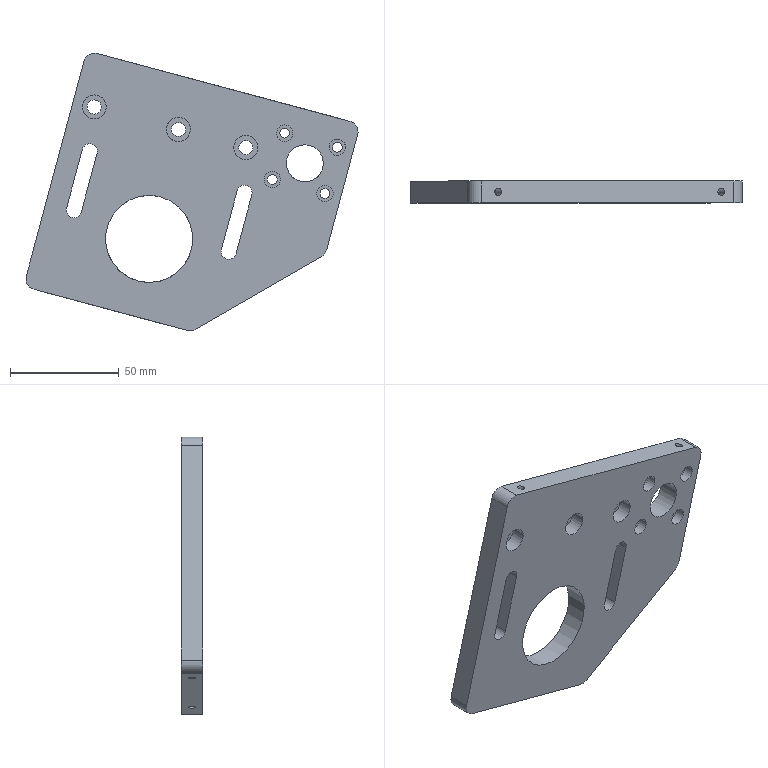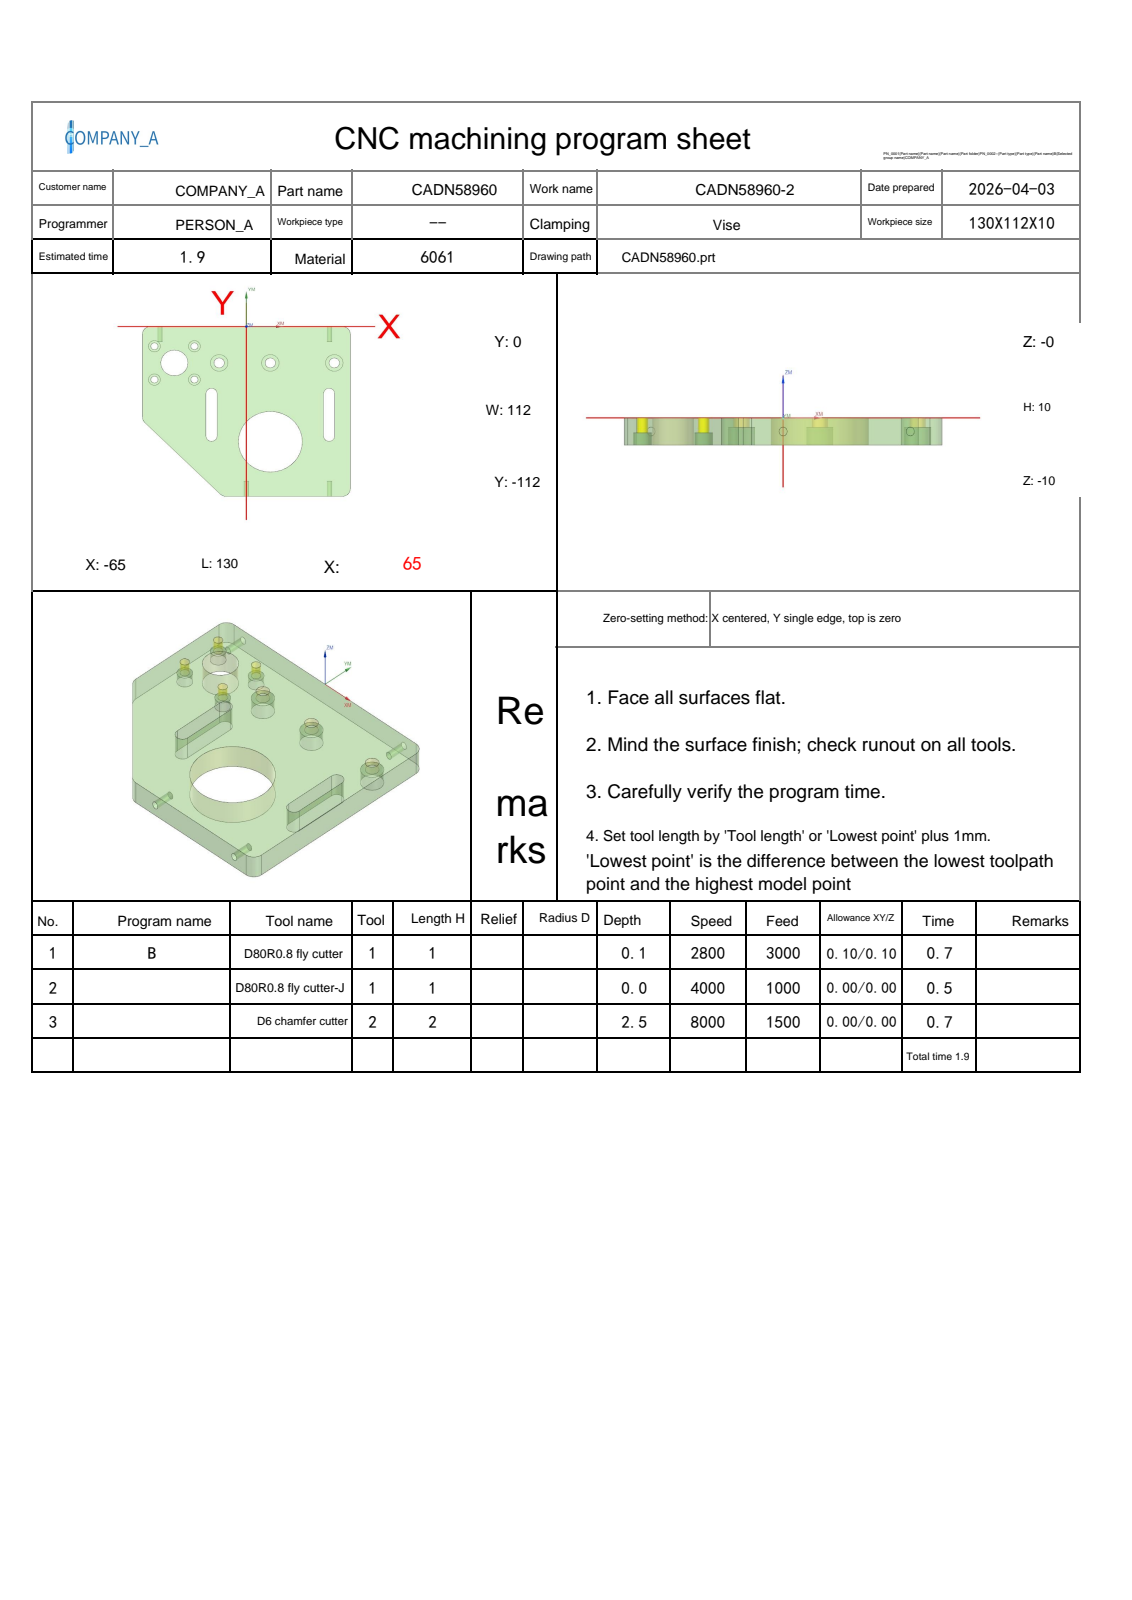NC program | NX | posted by the shop | part box 152.311 x 10 x 127.359 mm
Whole program:
%
O0001
(Machine time: 2.46 MIN)
(===Total Tool:2===)
(T1=D80R0.8 fly cutter D=80.  R=0.8  D-  H01 Z=-0.   )
(T2=D6 chamfer cutter   D=6.   R=0.   D-  H02 Z=-2.55 )
G80 G90 G17 G49 G40
G91 G28 Z0
M01
N1 T01 M06
(D80R0.8 fly cutter  D=80. R=0.8 H=01 ce=0.10 di=0.10)
G00 G90 G54 X117.097 Y-86.978 M03 S2800
G43 H01 Z20.
M08
Z3.525
G01 Z1.525 F3000.
X105.097 Y-87.213
X-88.772 Y-90.998
X-88.926 Y-90.999
G02 X-95.161 Y-88.011 I0.0 J8.
X-105.097 Y-59.772 I35.161 J28.239
G01 Y-39.991
G02 X-97.256 Y-31.996 I8. J-.003
G01 X105.097 Y-28.045
X117.097 Y-27.811
Z3.525
G00 Y-86.978
Z3.05
G01 Z1.05
X105.097 Y-87.213
X-88.772 Y-90.998
X-88.926 Y-90.999
G02 X-95.161 Y-88.011 I0.0 J8.
X-105.097 Y-59.772 I35.161 J28.239
G01 Y-39.991
G02 X-97.256 Y-31.996 I8. J-.003
G01 X105.097 Y-28.045
X117.097 Y-27.811
Z3.05
G00 Y-86.978
Z2.575
G01 Z.575
X105.097 Y-87.213
X-88.772 Y-90.998
X-88.926 Y-90.999
G02 X-95.161 Y-88.011 I0.0 J8.
X-105.097 Y-59.772 I35.161 J28.239
G01 Y-39.991
G02 X-97.256 Y-31.996 I8. J-.003
G01 X105.097 Y-28.045
X117.097 Y-27.811
Z2.575
G00 Y-86.978
Z2.1
G01 Z.1
X105.097 Y-87.213
X-88.772 Y-90.998
X-88.926 Y-90.999
G02 X-95.161 Y-88.011 I0.0 J8.
X-105.097 Y-59.772 I35.161 J28.239
G01 Y-39.991
G02 X-97.256 Y-31.996 I8. J-.003
G01 X105.097 Y-28.045
X117.097 Y-27.811
Z2.1
G00 Z20.
G91 G28 Z0.0
M05
M09
G91 G28 Z0.0
M01
N2 T01 M06
(D80R0.8 fly cutter-J  D=80. R=0.8 H=01 ce=0.00 di=0.00)
G00 G90 G54 X116.999 Y-86.884 M03 S4000
G43 H01 Z20.
M08
Z2.
G01 Z0.0 F1000.
X104.999 Y-87.118
X-88.729 Y-90.896
X-88.882 Y-90.897
G02 X-95.124 Y-87.9 I0.0 J8.
X-104.999 Y-59.772 I35.124 J28.128
G01 Y-40.087
G02 X-97.158 Y-32.091 I8. J-.003
G01 X104.999 Y-28.148
X116.999 Y-27.914
Z2.
G00 Z20.
G91 G28 Z0.0
M05
M09
G91 G28 Z0.0
M01
N3 T02 M06
(D6 chamfer cutter  D=6. R=0. H=02 ce=0.00 di=0.00)
G00 G90 G54 X-32.5 Y-35. M03 S8000
G43 H02 Z20.
M08
G98 G81 X-32.5 Y-35. Z-2.55 R3. F1000.
Y-13.
X-57.5
Y-35.
G80
G00 Z20.
G00 G90 X-.386 Y1.227 M03 S6500
Z20.
Z.172
G01 Z-1.499 F1500.
G03 X-.1 Y1.027 I1.286 J1.532
G01 X-.054 Y.997
X0.0 Y1.
X60.
G02 X66. Y-5. I0.0 J-6.
G01 Y-107.
G02 X60. Y-113. I-6. J0.0
G01 X-12.772
G02 X-17.015 Y-111.243 I0.0 J6.
G01 X-64.242 Y-64.015
G02 X-66. Y-59.772 I4.242 J4.243
G01 Y-5.
G02 X-60. Y1. I6. J0.0
G01 X0.0
X.054 Y.997
X.1 Y1.027
G03 X.386 Y1.227 I-1. J1.732
G01 Z.172
G00 Z10.
X9.759 Y-94.032
Z.198
G01 Z-1.499
G03 X9.991 Y-94.292 I1.602 J1.197
G01 X10.029 Y-94.332
X10.082 Y-94.341
G03 X15. Y-94.989 I4.918 J18.353
X34. Y-75.989 I0.0 J19.
X15. Y-56.989 I-19. J0.0
X-4. Y-75.989 I0.0 J-19.
X10.082 Y-94.341 I19. J0.0
G01 X10.134 Y-94.36
X10.186 Y-94.344
G03 X10.517 Y-94.235 I-.458 J1.947
G01 Z.194
G00 Z10.
X54.043 Y-58.605
Z.172
G01 Z-1.499
G03 X54.243 Y-58.319 I-1.532 J1.286
G01 X54.272 Y-58.273
X54.269 Y-58.219
Y-44.219
G03 X51.77 Y-41.719 I-2.5 J0.0
X49.27 Y-44.219 I0.0 J-2.5
G01 Y-72.219
G03 X51.77 Y-74.719 I2.5 J0.0
X54.269 Y-72.219 I0.0 J2.5
G01 Y-58.219
X54.272 Y-58.165
X54.243 Y-58.119
G03 X54.043 Y-57.834 I-1.732 J-1.
G01 Z.172
G00 Z10.
X54.077 Y-25.883
Z.253
G01 Z-1.499
G03 X54.324 Y-26.13 I1.532 J1.286
G01 X54.364 Y-26.167
X54.418 Y-26.173
G03 X55. Y-26.25 I.582 J2.173
X57.25 Y-24. I0.0 J2.25
X55. Y-21.75 I-2.25 J0.0
X52.75 Y-24. I0.0 J-2.25
X54.418 Y-26.173 I2.25 J0.0
G01 X54.468 Y-26.195
X54.521 Y-26.182
G03 X54.858 Y-26.092 I-.347 J1.97
G01 Z.254
G00 Z10.
X15.923 Y-22.117
Z.255
G01 Z-1.499
G03 X15.676 Y-21.87 I-1.532 J-1.286
G01 X15.636 Y-21.833
X15.582 Y-21.827
G03 X15. Y-21.75 I-.582 J-2.173
X12.75 Y-24. I0.0 J-2.25
X15. Y-26.25 I2.25 J0.0
X17.25 Y-24. I0.0 J2.25
X15.582 Y-21.827 I-2.25 J0.0
G01 X15.532 Y-21.805
X15.479 Y-21.818
G03 X15.142 Y-21.908 I.347 J-1.97
G01 Z.248
G00 Z10.
X-16.077 Y-22.117
Z.255
G01 Z-1.499
G03 X-16.324 Y-21.87 I-1.532 J-1.286
G01 X-16.364 Y-21.833
X-16.418 Y-21.827
G03 X-17. Y-21.75 I-.582 J-2.173
X-19.25 Y-24. I0.0 J-2.25
X-17. Y-26.25 I2.25 J0.0
X-14.75 Y-24. I0.0 J2.25
X-16.418 Y-21.827 I-2.25 J0.0
G01 X-16.468 Y-21.805
X-16.521 Y-21.818
G03 X-16.858 Y-21.908 I.347 J-1.97
G01 Z.248
G00 Z10.
X-33.169 Y-13.923
Z.295
G01 Z-1.499
G03 X-32.918 Y-14.165 I1.509 J1.312
G01 X-32.878 Y-14.202
X-32.824 Y-14.207
G03 X-32.5 Y-14.25 I.324 J1.207
X-31.25 Y-13. I0.0 J1.25
X-32.5 Y-11.75 I-1.25 J0.0
X-33.75 Y-13. I0.0 J-1.25
X-33.067 Y-14.114 I1.25 J0.0
G01 X-32.824 Y-14.207
X-32.774 Y-14.23
X-32.721 Y-14.218
G03 X-32.382 Y-14.134 I-.313 J1.975
G01 Z.294
G00 Z10.
X-47.27 Y-30.941
Z.209
G01 Z-1.499
G03 X-47.033 Y-31.197 I1.582 J1.224
G01 X-46.995 Y-31.236
X-46.941 Y-31.244
G03 X-45. Y-31.5 I1.941 J7.244
X-37.5 Y-24. I0.0 J7.5
X-45. Y-16.5 I-7.5 J0.0
X-52.5 Y-24. I0.0 J-7.5
X-46.941 Y-31.244 I7.5 J0.0
G01 X-46.89 Y-31.264
X-46.838 Y-31.249
G03 X-46.505 Y-31.146 I-.425 J1.954
G01 Z.21
G00 Z10.
X-58.169 Y-13.923
Z.295
G01 Z-1.499
G03 X-57.918 Y-14.165 I1.509 J1.312
G01 X-57.878 Y-14.202
X-57.824 Y-14.207
G03 X-57.5 Y-14.25 I.324 J1.207
X-56.25 Y-13. I0.0 J1.25
X-57.5 Y-11.75 I-1.25 J0.0
X-58.75 Y-13. I0.0 J-1.25
X-58.067 Y-14.114 I1.25 J0.0
G01 X-57.824 Y-14.207
X-57.774 Y-14.23
X-57.721 Y-14.218
G03 X-57.382 Y-14.134 I-.313 J1.975
G01 Z.294
G00 Z10.
X-56.831 Y-34.077
Z.295
G01 Z-1.499
G03 X-57.082 Y-33.835 I-1.509 J-1.312
G01 X-57.122 Y-33.798
X-57.176 Y-33.793
G03 X-57.5 Y-33.75 I-.324 J-1.207
X-58.75 Y-35. I0.0 J-1.25
X-57.5 Y-36.25 I1.25 J0.0
X-56.25 Y-35. I0.0 J1.25
X-56.933 Y-33.886 I-1.25 J0.0
G01 X-57.176 Y-33.793
X-57.226 Y-33.77
X-57.279 Y-33.782
G03 X-57.618 Y-33.866 I.313 J-1.975
G01 Z.294
G00 Z10.
X-33.169 Y-35.923
Z.295
G01 Z-1.499
G03 X-32.918 Y-36.165 I1.509 J1.312
G01 X-32.878 Y-36.202
X-32.824 Y-36.207
G03 X-32.5 Y-36.25 I.324 J1.207
X-31.25 Y-35. I0.0 J1.25
X-32.5 Y-33.75 I-1.25 J0.0
X-33.75 Y-35. I0.0 J-1.25
X-33.067 Y-36.114 I1.25 J0.0
G01 X-32.824 Y-36.207
X-32.774 Y-36.23
X-32.721 Y-36.218
G03 X-32.382 Y-36.134 I-.313 J1.975
G01 Z.294
G00 Z10.
X-19.496 Y-58.605
Z.172
G01 Z-1.499
G03 X-19.297 Y-58.319 I-1.532 J1.286
G01 X-19.267 Y-58.273
X-19.27 Y-58.219
Y-44.219
G03 X-21.77 Y-41.719 I-2.5 J0.0
X-24.269 Y-44.219 I0.0 J-2.5
G01 Y-72.219
G03 X-21.77 Y-74.719 I2.5 J0.0
X-19.27 Y-72.219 I0.0 J2.5
G01 Y-58.219
X-19.267 Y-58.165
X-19.297 Y-58.119
G03 X-19.496 Y-57.834 I-1.732 J-1.
G01 Z.172
G00 Z20.
M05
M09
G91 G28 Z0.0
G91 G28 Y0.0
M30
%